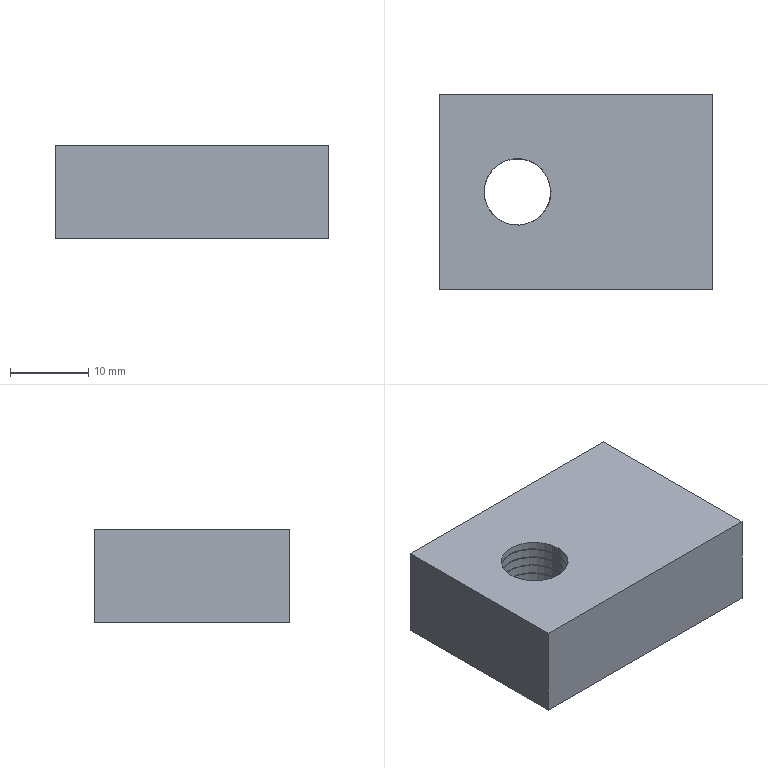Part | SolidWorks | features Extrusion 1, Helix 1, SweepCut 1 | 1 solid | 32 faces | box 35 x 25 x 12 mm | volume 9818 mm3 | cylinder 22 | plane 7 | spline 3 | commonest cylinder face diameters 8.5 x22